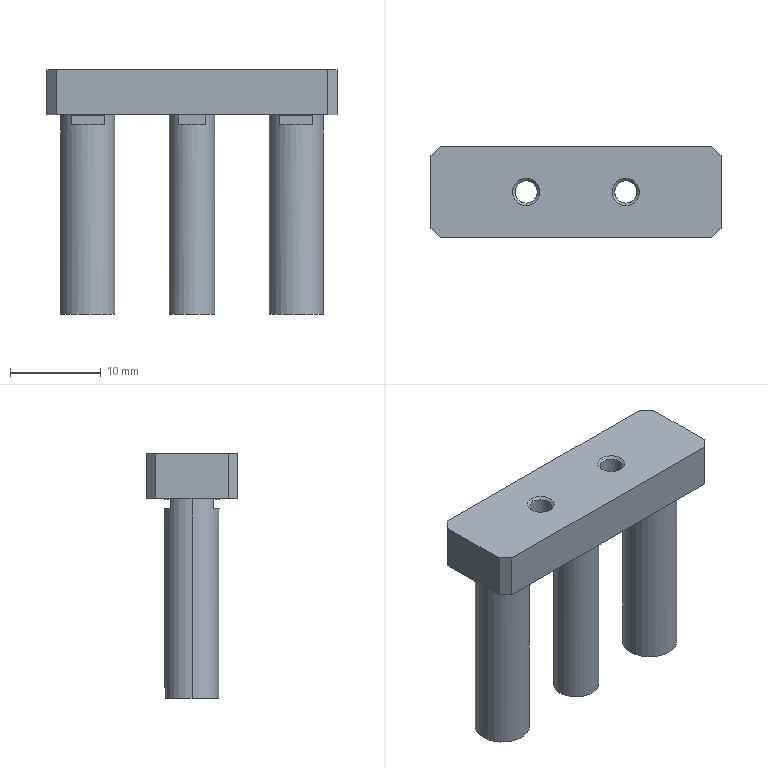Part | STEP file | MGJ10-20-F8NL2 | 1 solid | 47 faces | box 32 x 10 x 27 mm | volume 3209 mm3 | plane 29 | cylinder 10 | cone 8 | commonest cylinder face diameters 2.46 x4 6 x4 5 x2